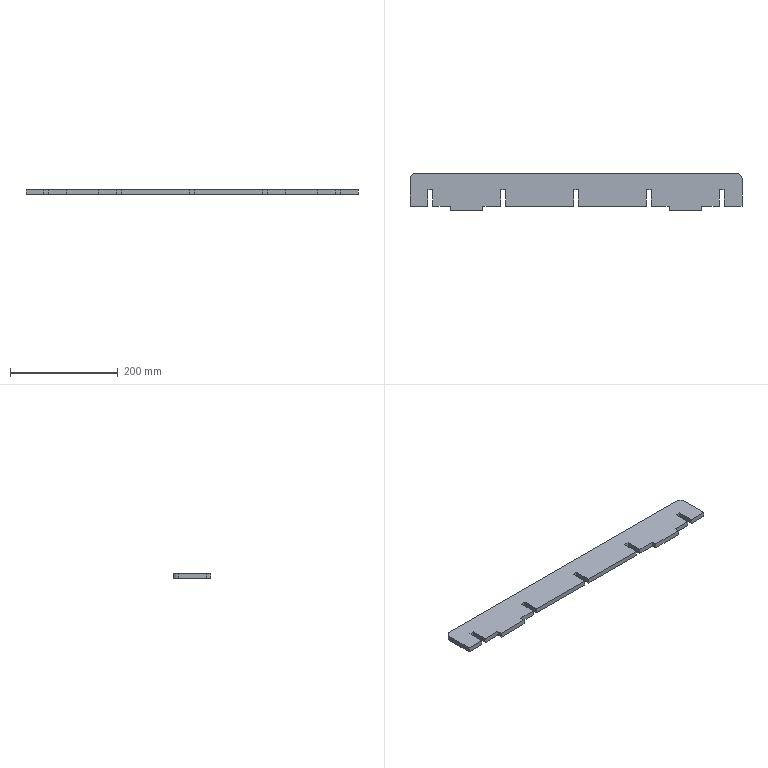Part | SolidWorks | features FlatPattern 1, SMBaseFlange 1, SheetMetal 1 | 1 solid | 36 faces | box 615 x 70 x 9 mm | volume 336641 mm3 | plane 34 | cylinder 2 | commonest cylinder face diameters 20 x2
STEP:
#1=CARTESIAN_POINT('',(336.887,-110.303,0.));
#2=VERTEX_POINT('',#1);
#3=CARTESIAN_POINT('',(369.887,-110.303,0.));
#4=VERTEX_POINT('',#3);
#5=CARTESIAN_POINT('',(336.887,-110.303,0.));
#6=DIRECTION('',(1.,0.,0.));
#7=VECTOR('',#6,1000.);
#8=LINE('',#5,#7);
#9=EDGE_CURVE('',#2,#4,#8,.T.);
#10=ORIENTED_EDGE('',*,*,#9,.F.);
#11=CARTESIAN_POINT('',(336.887,-110.303,-9.));
#12=VERTEX_POINT('',#11);
#13=CARTESIAN_POINT('',(336.887,-110.303,-9.));
#14=DIRECTION('',(0.,0.,1.));
#15=VECTOR('',#14,1000.);
#16=LINE('',#13,#15);
#17=EDGE_CURVE('',#12,#2,#16,.T.);
#18=ORIENTED_EDGE('',*,*,#17,.F.);
#19=CARTESIAN_POINT('',(369.887,-110.303,-9.));
#20=VERTEX_POINT('',#19);
#21=CARTESIAN_POINT('',(336.887,-110.303,-9.));
#22=DIRECTION('',(1.,0.,0.));
#23=VECTOR('',#22,1000.);
#24=LINE('',#21,#23);
#25=EDGE_CURVE('',#12,#20,#24,.T.);
#26=ORIENTED_EDGE('',*,*,#25,.T.);
#27=CARTESIAN_POINT('',(369.887,-110.303,-9.));
#28=DIRECTION('',(0.,0.,1.));
#29=VECTOR('',#28,1000.);
#30=LINE('',#27,#29);
#31=EDGE_CURVE('',#20,#4,#30,.T.);
#32=ORIENTED_EDGE('',*,*,#31,.T.);
#33=EDGE_LOOP('',(#10,#18,#26,#32));
#34=FACE_OUTER_BOUND('',#33,.T.);
#35=CARTESIAN_POINT('',(336.887,-110.303,-9.));
#36=DIRECTION('',(0.,-1.,0.));
#37=DIRECTION('',(1.,0.,0.));
#38=AXIS2_PLACEMENT_3D('',#35,#36,#37);
#39=PLANE('',#38);
#40=ADVANCED_FACE('',(#34),#39,.T.);
#41=CARTESIAN_POINT('',(336.887,-79.303,0.));
#42=VERTEX_POINT('',#41);
#43=CARTESIAN_POINT('',(336.887,-79.303,0.));
#44=DIRECTION('',(0.,-1.,0.));
#45=VECTOR('',#44,1000.);
#46=LINE('',#43,#45);
#47=EDGE_CURVE('',#42,#2,#46,.T.);
#48=ORIENTED_EDGE('',*,*,#47,.F.);
#49=CARTESIAN_POINT('',(336.887,-79.303,-9.));
#50=VERTEX_POINT('',#49);
#51=CARTESIAN_POINT('',(336.887,-79.303,-9.));
#52=DIRECTION('',(0.,0.,1.));
#53=VECTOR('',#52,1000.);
#54=LINE('',#51,#53);
#55=EDGE_CURVE('',#50,#42,#54,.T.);
#56=ORIENTED_EDGE('',*,*,#55,.F.);
#57=CARTESIAN_POINT('',(336.887,-79.303,-9.));
#58=DIRECTION('',(0.,-1.,0.));
#59=VECTOR('',#58,1000.);
#60=LINE('',#57,#59);
#61=EDGE_CURVE('',#50,#12,#60,.T.);
#62=ORIENTED_EDGE('',*,*,#61,.T.);
#63=ORIENTED_EDGE('',*,*,#17,.T.);
#64=EDGE_LOOP('',(#48,#56,#62,#63));
#65=FACE_OUTER_BOUND('',#64,.T.);
#66=CARTESIAN_POINT('',(336.887,-79.303,-9.));
#67=DIRECTION('',(-1.,0.,0.));
#68=DIRECTION('',(0.,0.,1.));
#69=AXIS2_PLACEMENT_3D('',#66,#67,#68);
#70=PLANE('',#69);
#71=ADVANCED_FACE('',(#65),#70,.T.);
#72=CARTESIAN_POINT('',(327.887,-79.303,0.));
#73=VERTEX_POINT('',#72);
#74=CARTESIAN_POINT('',(327.887,-79.303,0.));
#75=DIRECTION('',(1.,0.,0.));
#76=VECTOR('',#75,1000.);
#77=LINE('',#74,#76);
#78=EDGE_CURVE('',#73,#42,#77,.T.);
#79=ORIENTED_EDGE('',*,*,#78,.F.);
#80=CARTESIAN_POINT('',(327.887,-79.303,-9.));
#81=VERTEX_POINT('',#80);
#82=CARTESIAN_POINT('',(327.887,-79.303,-9.));
#83=DIRECTION('',(0.,0.,1.));
#84=VECTOR('',#83,1000.);
#85=LINE('',#82,#84);
#86=EDGE_CURVE('',#81,#73,#85,.T.);
#87=ORIENTED_EDGE('',*,*,#86,.F.);
#88=CARTESIAN_POINT('',(327.887,-79.303,-9.));
#89=DIRECTION('',(1.,0.,0.));
#90=VECTOR('',#89,1000.);
#91=LINE('',#88,#90);
#92=EDGE_CURVE('',#81,#50,#91,.T.);
#93=ORIENTED_EDGE('',*,*,#92,.T.);
#94=ORIENTED_EDGE('',*,*,#55,.T.);
#95=EDGE_LOOP('',(#79,#87,#93,#94));
#96=FACE_OUTER_BOUND('',#95,.T.);
#97=CARTESIAN_POINT('',(327.887,-79.303,-9.));
#98=DIRECTION('',(0.,-1.,0.));
#99=DIRECTION('',(0.,0.,-1.));
#100=AXIS2_PLACEMENT_3D('',#97,#98,#99);
#101=PLANE('',#100);
#102=ADVANCED_FACE('',(#96),#101,.T.);
#103=CARTESIAN_POINT('',(327.887,-110.303,0.));
#104=VERTEX_POINT('',#103);
#105=CARTESIAN_POINT('',(327.887,-110.303,0.));
#106=DIRECTION('',(0.,1.,0.));
#107=VECTOR('',#106,1000.);
#108=LINE('',#105,#107);
#109=EDGE_CURVE('',#104,#73,#108,.T.);
#110=ORIENTED_EDGE('',*,*,#109,.F.);
#111=CARTESIAN_POINT('',(327.887,-110.303,-9.));
#112=VERTEX_POINT('',#111);
#113=CARTESIAN_POINT('',(327.887,-110.303,-9.));
#114=DIRECTION('',(0.,0.,1.));
#115=VECTOR('',#114,1000.);
#116=LINE('',#113,#115);
#117=EDGE_CURVE('',#112,#104,#116,.T.);
#118=ORIENTED_EDGE('',*,*,#117,.F.);
#119=CARTESIAN_POINT('',(327.887,-110.303,-9.));
#120=DIRECTION('',(0.,1.,0.));
#121=VECTOR('',#120,1000.);
#122=LINE('',#119,#121);
#123=EDGE_CURVE('',#112,#81,#122,.T.);
#124=ORIENTED_EDGE('',*,*,#123,.T.);
#125=ORIENTED_EDGE('',*,*,#86,.T.);
#126=EDGE_LOOP('',(#110,#118,#124,#125));
#127=FACE_OUTER_BOUND('',#126,.T.);
#128=CARTESIAN_POINT('',(327.887,-110.303,-9.));
#129=DIRECTION('',(1.,0.,0.));
#130=DIRECTION('',(0.,1.,0.));
#131=AXIS2_PLACEMENT_3D('',#128,#129,#130);
#132=PLANE('',#131);
#133=ADVANCED_FACE('',(#127),#132,.T.);
#134=CARTESIAN_POINT('',(294.887,-110.303,0.));
#135=VERTEX_POINT('',#134);
#136=CARTESIAN_POINT('',(294.887,-110.303,0.));
#137=DIRECTION('',(1.,0.,0.));
#138=VECTOR('',#137,1000.);
#139=LINE('',#136,#138);
#140=EDGE_CURVE('',#135,#104,#139,.T.);
#141=ORIENTED_EDGE('',*,*,#140,.F.);
#142=CARTESIAN_POINT('',(294.887,-110.303,-9.));
#143=VERTEX_POINT('',#142);
#144=CARTESIAN_POINT('',(294.887,-110.303,-9.));
#145=DIRECTION('',(0.,0.,1.));
#146=VECTOR('',#145,1000.);
#147=LINE('',#144,#146);
#148=EDGE_CURVE('',#143,#135,#147,.T.);
#149=ORIENTED_EDGE('',*,*,#148,.F.);
#150=CARTESIAN_POINT('',(294.887,-110.303,-9.));
#151=DIRECTION('',(1.,0.,0.));
#152=VECTOR('',#151,1000.);
#153=LINE('',#150,#152);
#154=EDGE_CURVE('',#143,#112,#153,.T.);
#155=ORIENTED_EDGE('',*,*,#154,.T.);
#156=ORIENTED_EDGE('',*,*,#117,.T.);
#157=EDGE_LOOP('',(#141,#149,#155,#156));
#158=FACE_OUTER_BOUND('',#157,.T.);
#159=CARTESIAN_POINT('',(294.887,-110.303,-9.));
#160=DIRECTION('',(0.,-1.,0.));
#161=DIRECTION('',(1.,0.,0.));
#162=AXIS2_PLACEMENT_3D('',#159,#160,#161);
#163=PLANE('',#162);
#164=ADVANCED_FACE('',(#158),#163,.T.);
#165=CARTESIAN_POINT('',(294.887,-118.803,0.));
#166=VERTEX_POINT('',#165);
#167=CARTESIAN_POINT('',(294.887,-118.803,0.));
#168=DIRECTION('',(0.,1.,0.));
#169=VECTOR('',#168,1000.);
#170=LINE('',#167,#169);
#171=EDGE_CURVE('',#166,#135,#170,.T.);
#172=ORIENTED_EDGE('',*,*,#171,.F.);
#173=CARTESIAN_POINT('',(294.887,-118.803,-9.));
#174=VERTEX_POINT('',#173);
#175=CARTESIAN_POINT('',(294.887,-118.803,-9.));
#176=DIRECTION('',(0.,0.,1.));
#177=VECTOR('',#176,1000.);
#178=LINE('',#175,#177);
#179=EDGE_CURVE('',#174,#166,#178,.T.);
#180=ORIENTED_EDGE('',*,*,#179,.F.);
#181=CARTESIAN_POINT('',(294.887,-118.803,-9.));
#182=DIRECTION('',(0.,1.,0.));
#183=VECTOR('',#182,1000.);
#184=LINE('',#181,#183);
#185=EDGE_CURVE('',#174,#143,#184,.T.);
#186=ORIENTED_EDGE('',*,*,#185,.T.);
#187=ORIENTED_EDGE('',*,*,#148,.T.);
#188=EDGE_LOOP('',(#172,#180,#186,#187));
#189=FACE_OUTER_BOUND('',#188,.T.);
#190=CARTESIAN_POINT('',(294.887,-118.803,-9.));
#191=DIRECTION('',(1.,0.,0.));
#192=DIRECTION('',(0.,0.,-1.));
#193=AXIS2_PLACEMENT_3D('',#190,#191,#192);
#194=PLANE('',#193);
#195=ADVANCED_FACE('',(#189),#194,.T.);
#196=CARTESIAN_POINT('',(234.887,-118.803,0.));
#197=VERTEX_POINT('',#196);
#198=CARTESIAN_POINT('',(234.887,-118.803,0.));
#199=DIRECTION('',(1.,0.,0.));
#200=VECTOR('',#199,1000.);
#201=LINE('',#198,#200);
#202=EDGE_CURVE('',#197,#166,#201,.T.);
#203=ORIENTED_EDGE('',*,*,#202,.F.);
#204=CARTESIAN_POINT('',(234.887,-118.803,-9.));
#205=VERTEX_POINT('',#204);
#206=CARTESIAN_POINT('',(234.887,-118.803,-9.));
#207=DIRECTION('',(0.,0.,1.));
#208=VECTOR('',#207,1000.);
#209=LINE('',#206,#208);
#210=EDGE_CURVE('',#205,#197,#209,.T.);
#211=ORIENTED_EDGE('',*,*,#210,.F.);
#212=CARTESIAN_POINT('',(234.887,-118.803,-9.));
#213=DIRECTION('',(1.,0.,0.));
#214=VECTOR('',#213,1000.);
#215=LINE('',#212,#214);
#216=EDGE_CURVE('',#205,#174,#215,.T.);
#217=ORIENTED_EDGE('',*,*,#216,.T.);
#218=ORIENTED_EDGE('',*,*,#179,.T.);
#219=EDGE_LOOP('',(#203,#211,#217,#218));
#220=FACE_OUTER_BOUND('',#219,.T.);
#221=CARTESIAN_POINT('',(234.887,-118.803,-9.));
#222=DIRECTION('',(0.,-1.,0.));
#223=DIRECTION('',(0.,0.,-1.));
#224=AXIS2_PLACEMENT_3D('',#221,#222,#223);
#225=PLANE('',#224);
#226=ADVANCED_FACE('',(#220),#225,.T.);
#227=CARTESIAN_POINT('',(234.887,-110.303,0.));
#228=VERTEX_POINT('',#227);
#229=CARTESIAN_POINT('',(234.887,-110.303,0.));
#230=DIRECTION('',(0.,-1.,0.));
#231=VECTOR('',#230,1000.);
#232=LINE('',#229,#231);
#233=EDGE_CURVE('',#228,#197,#232,.T.);
#234=ORIENTED_EDGE('',*,*,#233,.F.);
#235=CARTESIAN_POINT('',(234.887,-110.303,-9.));
#236=VERTEX_POINT('',#235);
#237=CARTESIAN_POINT('',(234.887,-110.303,-9.));
#238=DIRECTION('',(0.,0.,1.));
#239=VECTOR('',#238,1000.);
#240=LINE('',#237,#239);
#241=EDGE_CURVE('',#236,#228,#240,.T.);
#242=ORIENTED_EDGE('',*,*,#241,.F.);
#243=CARTESIAN_POINT('',(234.887,-110.303,-9.));
#244=DIRECTION('',(0.,-1.,0.));
#245=VECTOR('',#244,1000.);
#246=LINE('',#243,#245);
#247=EDGE_CURVE('',#236,#205,#246,.T.);
#248=ORIENTED_EDGE('',*,*,#247,.T.);
#249=ORIENTED_EDGE('',*,*,#210,.T.);
#250=EDGE_LOOP('',(#234,#242,#248,#249));
#251=FACE_OUTER_BOUND('',#250,.T.);
#252=CARTESIAN_POINT('',(234.887,-110.303,-9.));
#253=DIRECTION('',(-1.,0.,0.));
#254=DIRECTION('',(0.,-1.,0.));
#255=AXIS2_PLACEMENT_3D('',#252,#253,#254);
#256=PLANE('',#255);
#257=ADVANCED_FACE('',(#251),#256,.T.);
#258=CARTESIAN_POINT('',(201.887,-110.303,0.));
#259=VERTEX_POINT('',#258);
#260=CARTESIAN_POINT('',(201.887,-110.303,0.));
#261=DIRECTION('',(1.,0.,0.));
#262=VECTOR('',#261,1000.);
#263=LINE('',#260,#262);
#264=EDGE_CURVE('',#259,#228,#263,.T.);
#265=ORIENTED_EDGE('',*,*,#264,.F.);
#266=CARTESIAN_POINT('',(201.887,-110.303,-9.));
#267=VERTEX_POINT('',#266);
#268=CARTESIAN_POINT('',(201.887,-110.303,-9.));
#269=DIRECTION('',(0.,0.,1.));
#270=VECTOR('',#269,1000.);
#271=LINE('',#268,#270);
#272=EDGE_CURVE('',#267,#259,#271,.T.);
#273=ORIENTED_EDGE('',*,*,#272,.F.);
#274=CARTESIAN_POINT('',(201.887,-110.303,-9.));
#275=DIRECTION('',(1.,0.,0.));
#276=VECTOR('',#275,1000.);
#277=LINE('',#274,#276);
#278=EDGE_CURVE('',#267,#236,#277,.T.);
#279=ORIENTED_EDGE('',*,*,#278,.T.);
#280=ORIENTED_EDGE('',*,*,#241,.T.);
#281=EDGE_LOOP('',(#265,#273,#279,#280));
#282=FACE_OUTER_BOUND('',#281,.T.);
#283=CARTESIAN_POINT('',(201.887,-110.303,-9.));
#284=DIRECTION('',(0.,-1.,0.));
#285=DIRECTION('',(1.,0.,0.));
#286=AXIS2_PLACEMENT_3D('',#283,#284,#285);
#287=PLANE('',#286);
#288=ADVANCED_FACE('',(#282),#287,.T.);
#289=CARTESIAN_POINT('',(201.887,-79.303,0.));
#290=VERTEX_POINT('',#289);
#291=CARTESIAN_POINT('',(201.887,-79.303,0.));
#292=DIRECTION('',(0.,-1.,0.));
#293=VECTOR('',#292,1000.);
#294=LINE('',#291,#293);
#295=EDGE_CURVE('',#290,#259,#294,.T.);
#296=ORIENTED_EDGE('',*,*,#295,.F.);
#297=CARTESIAN_POINT('',(201.887,-79.303,-9.));
#298=VERTEX_POINT('',#297);
#299=CARTESIAN_POINT('',(201.887,-79.303,-9.));
#300=DIRECTION('',(0.,0.,1.));
#301=VECTOR('',#300,1000.);
#302=LINE('',#299,#301);
#303=EDGE_CURVE('',#298,#290,#302,.T.);
#304=ORIENTED_EDGE('',*,*,#303,.F.);
#305=CARTESIAN_POINT('',(201.887,-79.303,-9.));
#306=DIRECTION('',(0.,-1.,0.));
#307=VECTOR('',#306,1000.);
#308=LINE('',#305,#307);
#309=EDGE_CURVE('',#298,#267,#308,.T.);
#310=ORIENTED_EDGE('',*,*,#309,.T.);
#311=ORIENTED_EDGE('',*,*,#272,.T.);
#312=EDGE_LOOP('',(#296,#304,#310,#311));
#313=FACE_OUTER_BOUND('',#312,.T.);
#314=CARTESIAN_POINT('',(201.887,-79.303,-9.));
#315=DIRECTION('',(-1.,0.,0.));
#316=DIRECTION('',(0.,0.,1.));
#317=AXIS2_PLACEMENT_3D('',#314,#315,#316);
#318=PLANE('',#317);
#319=ADVANCED_FACE('',(#313),#318,.T.);
#320=CARTESIAN_POINT('',(192.887,-79.303,0.));
#321=VERTEX_POINT('',#320);
#322=CARTESIAN_POINT('',(192.887,-79.303,0.));
#323=DIRECTION('',(1.,0.,0.));
#324=VECTOR('',#323,1000.);
#325=LINE('',#322,#324);
#326=EDGE_CURVE('',#321,#290,#325,.T.);
#327=ORIENTED_EDGE('',*,*,#326,.F.);
#328=CARTESIAN_POINT('',(192.887,-79.303,-9.));
#329=VERTEX_POINT('',#328);
#330=CARTESIAN_POINT('',(192.887,-79.303,-9.));
#331=DIRECTION('',(0.,0.,1.));
#332=VECTOR('',#331,1000.);
#333=LINE('',#330,#332);
#334=EDGE_CURVE('',#329,#321,#333,.T.);
#335=ORIENTED_EDGE('',*,*,#334,.F.);
#336=CARTESIAN_POINT('',(192.887,-79.303,-9.));
#337=DIRECTION('',(1.,0.,0.));
#338=VECTOR('',#337,1000.);
#339=LINE('',#336,#338);
#340=EDGE_CURVE('',#329,#298,#339,.T.);
#341=ORIENTED_EDGE('',*,*,#340,.T.);
#342=ORIENTED_EDGE('',*,*,#303,.T.);
#343=EDGE_LOOP('',(#327,#335,#341,#342));
#344=FACE_OUTER_BOUND('',#343,.T.);
#345=CARTESIAN_POINT('',(192.887,-79.303,-9.));
#346=DIRECTION('',(0.,-1.,0.));
#347=DIRECTION('',(0.,0.,-1.));
#348=AXIS2_PLACEMENT_3D('',#345,#346,#347);
#349=PLANE('',#348);
#350=ADVANCED_FACE('',(#344),#349,.T.);
#351=CARTESIAN_POINT('',(192.887,-110.303,0.));
#352=VERTEX_POINT('',#351);
#353=CARTESIAN_POINT('',(192.887,-110.303,0.));
#354=DIRECTION('',(0.,1.,0.));
#355=VECTOR('',#354,1000.);
#356=LINE('',#353,#355);
#357=EDGE_CURVE('',#352,#321,#356,.T.);
#358=ORIENTED_EDGE('',*,*,#357,.F.);
#359=CARTESIAN_POINT('',(192.887,-110.303,-9.));
#360=VERTEX_POINT('',#359);
#361=CARTESIAN_POINT('',(192.887,-110.303,-9.));
#362=DIRECTION('',(0.,0.,1.));
#363=VECTOR('',#362,1000.);
#364=LINE('',#361,#363);
#365=EDGE_CURVE('',#360,#352,#364,.T.);
#366=ORIENTED_EDGE('',*,*,#365,.F.);
#367=CARTESIAN_POINT('',(192.887,-110.303,-9.));
#368=DIRECTION('',(0.,1.,0.));
#369=VECTOR('',#368,1000.);
#370=LINE('',#367,#369);
#371=EDGE_CURVE('',#360,#329,#370,.T.);
#372=ORIENTED_EDGE('',*,*,#371,.T.);
#373=ORIENTED_EDGE('',*,*,#334,.T.);
#374=EDGE_LOOP('',(#358,#366,#372,#373));
#375=FACE_OUTER_BOUND('',#374,.T.);
#376=CARTESIAN_POINT('',(192.887,-110.303,-9.));
#377=DIRECTION('',(1.,0.,0.));
#378=DIRECTION('',(0.,1.,0.));
#379=AXIS2_PLACEMENT_3D('',#376,#377,#378);
#380=PLANE('',#379);
#381=ADVANCED_FACE('',(#375),#380,.T.);
#382=CARTESIAN_POINT('',(66.887,-110.303,0.));
#383=VERTEX_POINT('',#382);
#384=CARTESIAN_POINT('',(66.887,-110.303,0.));
#385=DIRECTION('',(1.,0.,0.));
#386=VECTOR('',#385,1000.);
#387=LINE('',#384,#386);
#388=EDGE_CURVE('',#383,#352,#387,.T.);
#389=ORIENTED_EDGE('',*,*,#388,.F.);
#390=CARTESIAN_POINT('',(66.887,-110.303,-9.));
#391=VERTEX_POINT('',#390);
#392=CARTESIAN_POINT('',(66.887,-110.303,-9.));
#393=DIRECTION('',(0.,0.,1.));
#394=VECTOR('',#393,1000.);
#395=LINE('',#392,#394);
#396=EDGE_CURVE('',#391,#383,#395,.T.);
#397=ORIENTED_EDGE('',*,*,#396,.F.);
#398=CARTESIAN_POINT('',(66.887,-110.303,-9.));
#399=DIRECTION('',(1.,0.,0.));
#400=VECTOR('',#399,1000.);
#401=LINE('',#398,#400);
#402=EDGE_CURVE('',#391,#360,#401,.T.);
#403=ORIENTED_EDGE('',*,*,#402,.T.);
#404=ORIENTED_EDGE('',*,*,#365,.T.);
#405=EDGE_LOOP('',(#389,#397,#403,#404));
#406=FACE_OUTER_BOUND('',#405,.T.);
#407=CARTESIAN_POINT('',(66.887,-110.303,-9.));
#408=DIRECTION('',(0.,-1.,0.));
#409=DIRECTION('',(1.,0.,0.));
#410=AXIS2_PLACEMENT_3D('',#407,#408,#409);
#411=PLANE('',#410);
#412=ADVANCED_FACE('',(#406),#411,.T.);
#413=CARTESIAN_POINT('',(66.887,-79.303,0.));
#414=VERTEX_POINT('',#413);
#415=CARTESIAN_POINT('',(66.887,-79.303,0.));
#416=DIRECTION('',(0.,-1.,0.));
#417=VECTOR('',#416,1000.);
#418=LINE('',#415,#417);
#419=EDGE_CURVE('',#414,#383,#418,.T.);
#420=ORIENTED_EDGE('',*,*,#419,.F.);
#421=CARTESIAN_POINT('',(66.887,-79.303,-9.));
#422=VERTEX_POINT('',#421);
#423=CARTESIAN_POINT('',(66.887,-79.303,-9.));
#424=DIRECTION('',(0.,0.,1.));
#425=VECTOR('',#424,1000.);
#426=LINE('',#423,#425);
#427=EDGE_CURVE('',#422,#414,#426,.T.);
#428=ORIENTED_EDGE('',*,*,#427,.F.);
#429=CARTESIAN_POINT('',(66.887,-79.303,-9.));
#430=DIRECTION('',(0.,-1.,0.));
#431=VECTOR('',#430,1000.);
#432=LINE('',#429,#431);
#433=EDGE_CURVE('',#422,#391,#432,.T.);
#434=ORIENTED_EDGE('',*,*,#433,.T.);
#435=ORIENTED_EDGE('',*,*,#396,.T.);
#436=EDGE_LOOP('',(#420,#428,#434,#435));
#437=FACE_OUTER_BOUND('',#436,.T.);
#438=CARTESIAN_POINT('',(66.887,-79.303,-9.));
#439=DIRECTION('',(-1.,0.,0.));
#440=DIRECTION('',(0.,0.,1.));
#441=AXIS2_PLACEMENT_3D('',#438,#439,#440);
#442=PLANE('',#441);
#443=ADVANCED_FACE('',(#437),#442,.T.);
#444=CARTESIAN_POINT('',(57.887,-79.303,0.));
#445=VERTEX_POINT('',#444);
#446=CARTESIAN_POINT('',(57.887,-79.303,0.));
#447=DIRECTION('',(1.,0.,0.));
#448=VECTOR('',#447,1000.);
#449=LINE('',#446,#448);
#450=EDGE_CURVE('',#445,#414,#449,.T.);
#451=ORIENTED_EDGE('',*,*,#450,.F.);
#452=CARTESIAN_POINT('',(57.887,-79.303,-9.));
#453=VERTEX_POINT('',#452);
#454=CARTESIAN_POINT('',(57.887,-79.303,-9.));
#455=DIRECTION('',(0.,0.,1.));
#456=VECTOR('',#455,1000.);
#457=LINE('',#454,#456);
#458=EDGE_CURVE('',#453,#445,#457,.T.);
#459=ORIENTED_EDGE('',*,*,#458,.F.);
#460=CARTESIAN_POINT('',(57.887,-79.303,-9.));
#461=DIRECTION('',(1.,0.,0.));
#462=VECTOR('',#461,1000.);
#463=LINE('',#460,#462);
#464=EDGE_CURVE('',#453,#422,#463,.T.);
#465=ORIENTED_EDGE('',*,*,#464,.T.);
#466=ORIENTED_EDGE('',*,*,#427,.T.);
#467=EDGE_LOOP('',(#451,#459,#465,#466));
#468=FACE_OUTER_BOUND('',#467,.T.);
#469=CARTESIAN_POINT('',(57.887,-79.303,-9.));
#470=DIRECTION('',(0.,-1.,0.));
#471=DIRECTION('',(0.,0.,-1.));
#472=AXIS2_PLACEMENT_3D('',#469,#470,#471);
#473=PLANE('',#472);
#474=ADVANCED_FACE('',(#468),#473,.T.);
#475=CARTESIAN_POINT('',(57.887,-110.303,0.));
#476=VERTEX_POINT('',#475);
#477=CARTESIAN_POINT('',(57.887,-110.303,0.));
#478=DIRECTION('',(0.,1.,0.));
#479=VECTOR('',#478,1000.);
#480=LINE('',#477,#479);
#481=EDGE_CURVE('',#476,#445,#480,.T.);
#482=ORIENTED_EDGE('',*,*,#481,.F.);
#483=CARTESIAN_POINT('',(57.887,-110.303,-9.));
#484=VERTEX_POINT('',#483);
#485=CARTESIAN_POINT('',(57.887,-110.303,-9.));
#486=DIRECTION('',(0.,0.,1.));
#487=VECTOR('',#486,1000.);
#488=LINE('',#485,#487);
#489=EDGE_CURVE('',#484,#476,#488,.T.);
#490=ORIENTED_EDGE('',*,*,#489,.F.);
#491=CARTESIAN_POINT('',(57.887,-110.303,-9.));
#492=DIRECTION('',(0.,1.,0.));
#493=VECTOR('',#492,1000.);
#494=LINE('',#491,#493);
#495=EDGE_CURVE('',#484,#453,#494,.T.);
#496=ORIENTED_EDGE('',*,*,#495,.T.);
#497=ORIENTED_EDGE('',*,*,#458,.T.);
#498=EDGE_LOOP('',(#482,#490,#496,#497));
#499=FACE_OUTER_BOUND('',#498,.T.);
#500=CARTESIAN_POINT('',(57.887,-110.303,-9.));
#501=DIRECTION('',(1.,0.,0.));
#502=DIRECTION('',(0.,0.,-1.));
#503=AXIS2_PLACEMENT_3D('',#500,#501,#502);
#504=PLANE('',#503);
#505=ADVANCED_FACE('',(#499),#504,.T.);
#506=CARTESIAN_POINT('',(-68.113,-110.303,0.));
#507=VERTEX_POINT('',#506);
#508=CARTESIAN_POINT('',(-68.113,-110.303,0.));
#509=DIRECTION('',(1.,0.,0.));
#510=VECTOR('',#509,1000.);
#511=LINE('',#508,#510);
#512=EDGE_CURVE('',#507,#476,#511,.T.);
#513=ORIENTED_EDGE('',*,*,#512,.F.);
#514=CARTESIAN_POINT('',(-68.113,-110.303,-9.));
#515=VERTEX_POINT('',#514);
#516=CARTESIAN_POINT('',(-68.113,-110.303,-9.));
#517=DIRECTION('',(0.,0.,1.));
#518=VECTOR('',#517,1000.);
#519=LINE('',#516,#518);
#520=EDGE_CURVE('',#515,#507,#519,.T.);
#521=ORIENTED_EDGE('',*,*,#520,.F.);
#522=CARTESIAN_POINT('',(-68.113,-110.303,-9.));
#523=DIRECTION('',(1.,0.,0.));
#524=VECTOR('',#523,1000.);
#525=LINE('',#522,#524);
#526=EDGE_CURVE('',#515,#484,#525,.T.);
#527=ORIENTED_EDGE('',*,*,#526,.T.);
#528=ORIENTED_EDGE('',*,*,#489,.T.);
#529=EDGE_LOOP('',(#513,#521,#527,#528));
#530=FACE_OUTER_BOUND('',#529,.T.);
#531=CARTESIAN_POINT('',(-68.113,-110.303,-9.));
#532=DIRECTION('',(0.,-1.,0.));
#533=DIRECTION('',(1.,0.,0.));
#534=AXIS2_PLACEMENT_3D('',#531,#532,#533);
#535=PLANE('',#534);
#536=ADVANCED_FACE('',(#530),#535,.T.);
#537=CARTESIAN_POINT('',(-68.113,-79.303,0.));
#538=VERTEX_POINT('',#537);
#539=CARTESIAN_POINT('',(-68.113,-79.303,0.));
#540=DIRECTION('',(0.,-1.,0.));
#541=VECTOR('',#540,1000.);
#542=LINE('',#539,#541);
#543=EDGE_CURVE('',#538,#507,#542,.T.);
#544=ORIENTED_EDGE('',*,*,#543,.F.);
#545=CARTESIAN_POINT('',(-68.113,-79.303,-9.));
#546=VERTEX_POINT('',#545);
#547=CARTESIAN_POINT('',(-68.113,-79.303,-9.));
#548=DIRECTION('',(0.,0.,1.));
#549=VECTOR('',#548,1000.);
#550=LINE('',#547,#549);
#551=EDGE_CURVE('',#546,#538,#550,.T.);
#552=ORIENTED_EDGE('',*,*,#551,.F.);
#553=CARTESIAN_POINT('',(-68.113,-79.303,-9.));
#554=DIRECTION('',(0.,-1.,0.));
#555=VECTOR('',#554,1000.);
#556=LINE('',#553,#555);
#557=EDGE_CURVE('',#546,#515,#556,.T.);
#558=ORIENTED_EDGE('',*,*,#557,.T.);
#559=ORIENTED_EDGE('',*,*,#520,.T.);
#560=EDGE_LOOP('',(#544,#552,#558,#559));
#561=FACE_OUTER_BOUND('',#560,.T.);
#562=CARTESIAN_POINT('',(-68.113,-79.303,-9.));
#563=DIRECTION('',(-1.,0.,0.));
#564=DIRECTION('',(0.,0.,1.));
#565=AXIS2_PLACEMENT_3D('',#562,#563,#564);
#566=PLANE('',#565);
#567=ADVANCED_FACE('',(#561),#566,.T.);
#568=CARTESIAN_POINT('',(-77.113,-79.303,0.));
#569=VERTEX_POINT('',#568);
#570=CARTESIAN_POINT('',(-77.113,-79.303,0.));
#571=DIRECTION('',(1.,0.,0.));
#572=VECTOR('',#571,1000.);
#573=LINE('',#570,#572);
#574=EDGE_CURVE('',#569,#538,#573,.T.);
#575=ORIENTED_EDGE('',*,*,#574,.F.);
#576=CARTESIAN_POINT('',(-77.113,-79.303,-9.));
#577=VERTEX_POINT('',#576);
#578=CARTESIAN_POINT('',(-77.113,-79.303,-9.));
#579=DIRECTION('',(0.,0.,1.));
#580=VECTOR('',#579,1000.);
#581=LINE('',#578,#580);
#582=EDGE_CURVE('',#577,#569,#581,.T.);
#583=ORIENTED_EDGE('',*,*,#582,.F.);
#584=CARTESIAN_POINT('',(-77.113,-79.303,-9.));
#585=DIRECTION('',(1.,0.,0.));
#586=VECTOR('',#585,1000.);
#587=LINE('',#584,#586);
#588=EDGE_CURVE('',#577,#546,#587,.T.);
#589=ORIENTED_EDGE('',*,*,#588,.T.);
#590=ORIENTED_EDGE('',*,*,#551,.T.);
#591=EDGE_LOOP('',(#575,#583,#589,#590));
#592=FACE_OUTER_BOUND('',#591,.T.);
#593=CARTESIAN_POINT('',(-77.113,-79.303,-9.));
#594=DIRECTION('',(0.,-1.,0.));
#595=DIRECTION('',(0.,0.,-1.));
#596=AXIS2_PLACEMENT_3D('',#593,#594,#595);
#597=PLANE('',#596);
#598=ADVANCED_FACE('',(#592),#597,.T.);
#599=CARTESIAN_POINT('',(-77.113,-110.303,0.));
#600=VERTEX_POINT('',#599);
#601=CARTESIAN_POINT('',(-77.113,-110.303,0.));
#602=DIRECTION('',(0.,1.,0.));
#603=VECTOR('',#602,1000.);
#604=LINE('',#601,#603);
#605=EDGE_CURVE('',#600,#569,#604,.T.);
#606=ORIENTED_EDGE('',*,*,#605,.F.);
#607=CARTESIAN_POINT('',(-77.113,-110.303,-9.));
#608=VERTEX_POINT('',#607);
#609=CARTESIAN_POINT('',(-77.113,-110.303,-9.));
#610=DIRECTION('',(0.,0.,1.));
#611=VECTOR('',#610,1000.);
#612=LINE('',#609,#611);
#613=EDGE_CURVE('',#608,#600,#612,.T.);
#614=ORIENTED_EDGE('',*,*,#613,.F.);
#615=CARTESIAN_POINT('',(-77.113,-110.303,-9.));
#616=DIRECTION('',(0.,1.,0.));
#617=VECTOR('',#616,1000.);
#618=LINE('',#615,#617);
#619=EDGE_CURVE('',#608,#577,#618,.T.);
#620=ORIENTED_EDGE('',*,*,#619,.T.);
#621=ORIENTED_EDGE('',*,*,#582,.T.);
#622=EDGE_LOOP('',(#606,#614,#620,#621));
#623=FACE_OUTER_BOUND('',#622,.T.);
#624=CARTESIAN_POINT('',(-77.113,-110.303,-9.));
#625=DIRECTION('',(1.,0.,0.));
#626=DIRECTION('',(0.,1.,0.));
#627=AXIS2_PLACEMENT_3D('',#624,#625,#626);
#628=PLANE('',#627);
#629=ADVANCED_FACE('',(#623),#628,.T.);
#630=CARTESIAN_POINT('',(-110.113,-110.303,0.));
#631=VERTEX_POINT('',#630);
#632=CARTESIAN_POINT('',(-110.113,-110.303,0.));
#633=DIRECTION('',(1.,0.,0.));
#634=VECTOR('',#633,1000.);
#635=LINE('',#632,#634);
#636=EDGE_CURVE('',#631,#600,#635,.T.);
#637=ORIENTED_EDGE('',*,*,#636,.F.);
#638=CARTESIAN_POINT('',(-110.113,-110.303,-9.));
#639=VERTEX_POINT('',#638);
#640=CARTESIAN_POINT('',(-110.113,-110.303,-9.));
#641=DIRECTION('',(0.,0.,1.));
#642=VECTOR('',#641,1000.);
#643=LINE('',#640,#642);
#644=EDGE_CURVE('',#639,#631,#643,.T.);
#645=ORIENTED_EDGE('',*,*,#644,.F.);
#646=CARTESIAN_POINT('',(-110.113,-110.303,-9.));
#647=DIRECTION('',(1.,0.,0.));
#648=VECTOR('',#647,1000.);
#649=LINE('',#646,#648);
#650=EDGE_CURVE('',#639,#608,#649,.T.);
#651=ORIENTED_EDGE('',*,*,#650,.T.);
#652=ORIENTED_EDGE('',*,*,#613,.T.);
#653=EDGE_LOOP('',(#637,#645,#651,#652));
#654=FACE_OUTER_BOUND('',#653,.T.);
#655=CARTESIAN_POINT('',(-110.113,-110.303,-9.));
#656=DIRECTION('',(0.,-1.,0.));
#657=DIRECTION('',(1.,0.,0.));
#658=AXIS2_PLACEMENT_3D('',#655,#656,#657);
#659=PLANE('',#658);
#660=ADVANCED_FACE('',(#654),#659,.T.);
#661=CARTESIAN_POINT('',(-110.113,-118.803,0.));
#662=VERTEX_POINT('',#661);
#663=CARTESIAN_POINT('',(-110.113,-118.803,0.));
#664=DIRECTION('',(0.,1.,0.));
#665=VECTOR('',#664,1000.);
#666=LINE('',#663,#665);
#667=EDGE_CURVE('',#662,#631,#666,.T.);
#668=ORIENTED_EDGE('',*,*,#667,.F.);
#669=CARTESIAN_POINT('',(-110.113,-118.803,-9.));
#670=VERTEX_POINT('',#669);
#671=CARTESIAN_POINT('',(-110.113,-118.803,-9.));
#672=DIRECTION('',(0.,0.,1.));
#673=VECTOR('',#672,1000.);
#674=LINE('',#671,#673);
#675=EDGE_CURVE('',#670,#662,#674,.T.);
#676=ORIENTED_EDGE('',*,*,#675,.F.);
#677=CARTESIAN_POINT('',(-110.113,-118.803,-9.));
#678=DIRECTION('',(0.,1.,0.));
#679=VECTOR('',#678,1000.);
#680=LINE('',#677,#679);
#681=EDGE_CURVE('',#670,#639,#680,.T.);
#682=ORIENTED_EDGE('',*,*,#681,.T.);
#683=ORIENTED_EDGE('',*,*,#644,.T.);
#684=EDGE_LOOP('',(#668,#676,#682,#683));
#685=FACE_OUTER_BOUND('',#684,.T.);
#686=CARTESIAN_POINT('',(-110.113,-118.803,-9.));
#687=DIRECTION('',(1.,0.,0.));
#688=DIRECTION('',(0.,0.,-1.));
#689=AXIS2_PLACEMENT_3D('',#686,#687,#688);
#690=PLANE('',#689);
#691=ADVANCED_FACE('',(#685),#690,.T.);
#692=CARTESIAN_POINT('',(-170.113,-118.803,0.));
#693=VERTEX_POINT('',#692);
#694=CARTESIAN_POINT('',(-170.113,-118.803,0.));
#695=DIRECTION('',(1.,0.,0.));
#696=VECTOR('',#695,1000.);
#697=LINE('',#694,#696);
#698=EDGE_CURVE('',#693,#662,#697,.T.);
#699=ORIENTED_EDGE('',*,*,#698,.F.);
#700=CARTESIAN_POINT('',(-170.113,-118.803,-9.));
#701=VERTEX_POINT('',#700);
#702=CARTESIAN_POINT('',(-170.113,-118.803,-9.));
#703=DIRECTION('',(0.,0.,1.));
#704=VECTOR('',#703,1000.);
#705=LINE('',#702,#704);
#706=EDGE_CURVE('',#701,#693,#705,.T.);
#707=ORIENTED_EDGE('',*,*,#706,.F.);
#708=CARTESIAN_POINT('',(-170.113,-118.803,-9.));
#709=DIRECTION('',(1.,0.,0.));
#710=VECTOR('',#709,1000.);
#711=LINE('',#708,#710);
#712=EDGE_CURVE('',#701,#670,#711,.T.);
#713=ORIENTED_EDGE('',*,*,#712,.T.);
#714=ORIENTED_EDGE('',*,*,#675,.T.);
#715=EDGE_LOOP('',(#699,#707,#713,#714));
#716=FACE_OUTER_BOUND('',#715,.T.);
#717=CARTESIAN_POINT('',(-170.113,-118.803,-9.));
#718=DIRECTION('',(0.,-1.,0.));
#719=DIRECTION('',(0.,0.,-1.));
#720=AXIS2_PLACEMENT_3D('',#717,#718,#719);
#721=PLANE('',#720);
#722=ADVANCED_FACE('',(#716),#721,.T.);
#723=CARTESIAN_POINT('',(-170.113,-110.303,0.));
#724=VERTEX_POINT('',#723);
#725=CARTESIAN_POINT('',(-170.113,-110.303,0.));
#726=DIRECTION('',(0.,-1.,0.));
#727=VECTOR('',#726,1000.);
#728=LINE('',#725,#727);
#729=EDGE_CURVE('',#724,#693,#728,.T.);
#730=ORIENTED_EDGE('',*,*,#729,.F.);
#731=CARTESIAN_POINT('',(-170.113,-110.303,-9.));
#732=VERTEX_POINT('',#731);
#733=CARTESIAN_POINT('',(-170.113,-110.303,-9.));
#734=DIRECTION('',(0.,0.,1.));
#735=VECTOR('',#734,1000.);
#736=LINE('',#733,#735);
#737=EDGE_CURVE('',#732,#724,#736,.T.);
#738=ORIENTED_EDGE('',*,*,#737,.F.);
#739=CARTESIAN_POINT('',(-170.113,-110.303,-9.));
#740=DIRECTION('',(0.,-1.,0.));
#741=VECTOR('',#740,1000.);
#742=LINE('',#739,#741);
#743=EDGE_CURVE('',#732,#701,#742,.T.);
#744=ORIENTED_EDGE('',*,*,#743,.T.);
#745=ORIENTED_EDGE('',*,*,#706,.T.);
#746=EDGE_LOOP('',(#730,#738,#744,#745));
#747=FACE_OUTER_BOUND('',#746,.T.);
#748=CARTESIAN_POINT('',(-170.113,-110.303,-9.));
#749=DIRECTION('',(-1.,0.,0.));
#750=DIRECTION('',(0.,0.,1.));
#751=AXIS2_PLACEMENT_3D('',#748,#749,#750);
#752=PLANE('',#751);
#753=ADVANCED_FACE('',(#747),#752,.T.);
#754=CARTESIAN_POINT('',(-203.113,-110.303,0.));
#755=VERTEX_POINT('',#754);
#756=CARTESIAN_POINT('',(-203.113,-110.303,0.));
#757=DIRECTION('',(1.,0.,0.));
#758=VECTOR('',#757,1000.);
#759=LINE('',#756,#758);
#760=EDGE_CURVE('',#755,#724,#759,.T.);
#761=ORIENTED_EDGE('',*,*,#760,.F.);
#762=CARTESIAN_POINT('',(-203.113,-110.303,-9.));
#763=VERTEX_POINT('',#762);
#764=CARTESIAN_POINT('',(-203.113,-110.303,-9.));
#765=DIRECTION('',(0.,0.,1.));
#766=VECTOR('',#765,1000.);
#767=LINE('',#764,#766);
#768=EDGE_CURVE('',#763,#755,#767,.T.);
#769=ORIENTED_EDGE('',*,*,#768,.F.);
#770=CARTESIAN_POINT('',(-203.113,-110.303,-9.));
#771=DIRECTION('',(1.,0.,0.));
#772=VECTOR('',#771,1000.);
#773=LINE('',#770,#772);
#774=EDGE_CURVE('',#763,#732,#773,.T.);
#775=ORIENTED_EDGE('',*,*,#774,.T.);
#776=ORIENTED_EDGE('',*,*,#737,.T.);
#777=EDGE_LOOP('',(#761,#769,#775,#776));
#778=FACE_OUTER_BOUND('',#777,.T.);
#779=CARTESIAN_POINT('',(-203.113,-110.303,-9.));
#780=DIRECTION('',(0.,-1.,0.));
#781=DIRECTION('',(1.,0.,0.));
#782=AXIS2_PLACEMENT_3D('',#779,#780,#781);
#783=PLANE('',#782);
#784=ADVANCED_FACE('',(#778),#783,.T.);
#785=CARTESIAN_POINT('',(-203.113,-79.303,0.));
#786=VERTEX_POINT('',#785);
#787=CARTESIAN_POINT('',(-203.113,-79.303,0.));
#788=DIRECTION('',(0.,-1.,0.));
#789=VECTOR('',#788,1000.);
#790=LINE('',#787,#789);
#791=EDGE_CURVE('',#786,#755,#790,.T.);
#792=ORIENTED_EDGE('',*,*,#791,.F.);
#793=CARTESIAN_POINT('',(-203.113,-79.303,-9.));
#794=VERTEX_POINT('',#793);
#795=CARTESIAN_POINT('',(-203.113,-79.303,-9.));
#796=DIRECTION('',(0.,0.,1.));
#797=VECTOR('',#796,1000.);
#798=LINE('',#795,#797);
#799=EDGE_CURVE('',#794,#786,#798,.T.);
#800=ORIENTED_EDGE('',*,*,#799,.F.);
#801=CARTESIAN_POINT('',(-203.113,-79.303,-9.));
#802=DIRECTION('',(0.,-1.,0.));
#803=VECTOR('',#802,1000.);
#804=LINE('',#801,#803);
#805=EDGE_CURVE('',#794,#763,#804,.T.);
#806=ORIENTED_EDGE('',*,*,#805,.T.);
#807=ORIENTED_EDGE('',*,*,#768,.T.);
#808=EDGE_LOOP('',(#792,#800,#806,#807));
#809=FACE_OUTER_BOUND('',#808,.T.);
#810=CARTESIAN_POINT('',(-203.113,-79.303,-9.));
#811=DIRECTION('',(-1.,0.,0.));
#812=DIRECTION('',(0.,0.,1.));
#813=AXIS2_PLACEMENT_3D('',#810,#811,#812);
#814=PLANE('',#813);
#815=ADVANCED_FACE('',(#809),#814,.T.);
#816=CARTESIAN_POINT('',(-212.113,-79.303,0.));
#817=VERTEX_POINT('',#816);
#818=CARTESIAN_POINT('',(-212.113,-79.303,0.));
#819=DIRECTION('',(1.,0.,0.));
#820=VECTOR('',#819,1000.);
#821=LINE('',#818,#820);
#822=EDGE_CURVE('',#817,#786,#821,.T.);
#823=ORIENTED_EDGE('',*,*,#822,.F.);
#824=CARTESIAN_POINT('',(-212.113,-79.303,-9.));
#825=VERTEX_POINT('',#824);
#826=CARTESIAN_POINT('',(-212.113,-79.303,-9.));
#827=DIRECTION('',(0.,0.,1.));
#828=VECTOR('',#827,1000.);
#829=LINE('',#826,#828);
#830=EDGE_CURVE('',#825,#817,#829,.T.);
#831=ORIENTED_EDGE('',*,*,#830,.F.);
#832=CARTESIAN_POINT('',(-212.113,-79.303,-9.));
#833=DIRECTION('',(1.,0.,0.));
#834=VECTOR('',#833,1000.);
#835=LINE('',#832,#834);
#836=EDGE_CURVE('',#825,#794,#835,.T.);
#837=ORIENTED_EDGE('',*,*,#836,.T.);
#838=ORIENTED_EDGE('',*,*,#799,.T.);
#839=EDGE_LOOP('',(#823,#831,#837,#838));
#840=FACE_OUTER_BOUND('',#839,.T.);
#841=CARTESIAN_POINT('',(-212.113,-79.303,-9.));
#842=DIRECTION('',(0.,-1.,0.));
#843=DIRECTION('',(0.,0.,-1.));
#844=AXIS2_PLACEMENT_3D('',#841,#842,#843);
#845=PLANE('',#844);
#846=ADVANCED_FACE('',(#840),#845,.T.);
#847=CARTESIAN_POINT('',(-212.113,-110.303,0.));
#848=VERTEX_POINT('',#847);
#849=CARTESIAN_POINT('',(-212.113,-110.303,0.));
#850=DIRECTION('',(0.,1.,0.));
#851=VECTOR('',#850,1000.);
#852=LINE('',#849,#851);
#853=EDGE_CURVE('',#848,#817,#852,.T.);
#854=ORIENTED_EDGE('',*,*,#853,.F.);
#855=CARTESIAN_POINT('',(-212.113,-110.303,-9.));
#856=VERTEX_POINT('',#855);
#857=CARTESIAN_POINT('',(-212.113,-110.303,-9.));
#858=DIRECTION('',(0.,0.,1.));
#859=VECTOR('',#858,1000.);
#860=LINE('',#857,#859);
#861=EDGE_CURVE('',#856,#848,#860,.T.);
#862=ORIENTED_EDGE('',*,*,#861,.F.);
#863=CARTESIAN_POINT('',(-212.113,-110.303,-9.));
#864=DIRECTION('',(0.,1.,0.));
#865=VECTOR('',#864,1000.);
#866=LINE('',#863,#865);
#867=EDGE_CURVE('',#856,#825,#866,.T.);
#868=ORIENTED_EDGE('',*,*,#867,.T.);
#869=ORIENTED_EDGE('',*,*,#830,.T.);
#870=EDGE_LOOP('',(#854,#862,#868,#869));
#871=FACE_OUTER_BOUND('',#870,.T.);
#872=CARTESIAN_POINT('',(-212.113,-110.303,-9.));
#873=DIRECTION('',(1.,0.,0.));
#874=DIRECTION('',(0.,0.,-1.));
#875=AXIS2_PLACEMENT_3D('',#872,#873,#874);
#876=PLANE('',#875);
#877=ADVANCED_FACE('',(#871),#876,.T.);
#878=CARTESIAN_POINT('',(-245.113,-110.303,0.));
#879=VERTEX_POINT('',#878);
#880=CARTESIAN_POINT('',(-245.113,-110.303,0.));
#881=DIRECTION('',(1.,0.,0.));
#882=VECTOR('',#881,1000.);
#883=LINE('',#880,#882);
#884=EDGE_CURVE('',#879,#848,#883,.T.);
#885=ORIENTED_EDGE('',*,*,#884,.F.);
#886=CARTESIAN_POINT('',(-245.113,-110.303,-9.));
#887=VERTEX_POINT('',#886);
#888=CARTESIAN_POINT('',(-245.113,-110.303,-9.));
#889=DIRECTION('',(0.,0.,1.));
#890=VECTOR('',#889,1000.);
#891=LINE('',#888,#890);
#892=EDGE_CURVE('',#887,#879,#891,.T.);
#893=ORIENTED_EDGE('',*,*,#892,.F.);
#894=CARTESIAN_POINT('',(-245.113,-110.303,-9.));
#895=DIRECTION('',(1.,0.,0.));
#896=VECTOR('',#895,1000.);
#897=LINE('',#894,#896);
#898=EDGE_CURVE('',#887,#856,#897,.T.);
#899=ORIENTED_EDGE('',*,*,#898,.T.);
#900=ORIENTED_EDGE('',*,*,#861,.T.);
#901=EDGE_LOOP('',(#885,#893,#899,#900));
#902=FACE_OUTER_BOUND('',#901,.T.);
#903=CARTESIAN_POINT('',(-245.113,-110.303,-9.));
#904=DIRECTION('',(0.,-1.,0.));
#905=DIRECTION('',(1.,0.,0.));
#906=AXIS2_PLACEMENT_3D('',#903,#904,#905);
#907=PLANE('',#906);
#908=ADVANCED_FACE('',(#902),#907,.T.);
#909=CARTESIAN_POINT('',(-245.113,-58.803,0.));
#910=VERTEX_POINT('',#909);
#911=CARTESIAN_POINT('',(-245.113,-58.803,0.));
#912=DIRECTION('',(0.,-1.,0.));
#913=VECTOR('',#912,1000.);
#914=LINE('',#911,#913);
#915=EDGE_CURVE('',#910,#879,#914,.T.);
#916=ORIENTED_EDGE('',*,*,#915,.F.);
#917=CARTESIAN_POINT('',(-245.113,-58.803,-9.));
#918=VERTEX_POINT('',#917);
#919=CARTESIAN_POINT('',(-245.113,-58.803,-9.));
#920=DIRECTION('',(0.,0.,1.));
#921=VECTOR('',#920,1000.);
#922=LINE('',#919,#921);
#923=EDGE_CURVE('',#918,#910,#922,.T.);
#924=ORIENTED_EDGE('',*,*,#923,.F.);
#925=CARTESIAN_POINT('',(-245.113,-58.803,-9.));
#926=DIRECTION('',(0.,-1.,0.));
#927=VECTOR('',#926,1000.);
#928=LINE('',#925,#927);
#929=EDGE_CURVE('',#918,#887,#928,.T.);
#930=ORIENTED_EDGE('',*,*,#929,.T.);
#931=ORIENTED_EDGE('',*,*,#892,.T.);
#932=EDGE_LOOP('',(#916,#924,#930,#931));
#933=FACE_OUTER_BOUND('',#932,.T.);
#934=CARTESIAN_POINT('',(-245.113,-58.803,-9.));
#935=DIRECTION('',(-1.,0.,0.));
#936=DIRECTION('',(0.,0.,1.));
#937=AXIS2_PLACEMENT_3D('',#934,#935,#936);
#938=PLANE('',#937);
#939=ADVANCED_FACE('',(#933),#938,.T.);
#940=CARTESIAN_POINT('',(-235.113,-48.803,0.));
#941=VERTEX_POINT('',#940);
#942=CARTESIAN_POINT('',(-235.113,-58.803,0.));
#943=DIRECTION('',(0.,0.,1.));
#944=DIRECTION('',(1.,0.,0.));
#945=AXIS2_PLACEMENT_3D('',#942,#943,#944);
#946=CIRCLE('',#945,10.);
#947=EDGE_CURVE('',#941,#910,#946,.T.);
#948=ORIENTED_EDGE('',*,*,#947,.F.);
#949=CARTESIAN_POINT('',(-235.113,-48.803,-9.));
#950=VERTEX_POINT('',#949);
#951=CARTESIAN_POINT('',(-235.113,-48.803,-9.));
#952=DIRECTION('',(0.,0.,1.));
#953=VECTOR('',#952,1000.);
#954=LINE('',#951,#953);
#955=EDGE_CURVE('',#950,#941,#954,.T.);
#956=ORIENTED_EDGE('',*,*,#955,.F.);
#957=CARTESIAN_POINT('',(-235.113,-58.803,-9.));
#958=DIRECTION('',(0.,0.,1.));
#959=DIRECTION('',(1.,0.,0.));
#960=AXIS2_PLACEMENT_3D('',#957,#958,#959);
#961=CIRCLE('',#960,10.);
#962=EDGE_CURVE('',#950,#918,#961,.T.);
#963=ORIENTED_EDGE('',*,*,#962,.T.);
#964=ORIENTED_EDGE('',*,*,#923,.T.);
#965=EDGE_LOOP('',(#948,#956,#963,#964));
#966=FACE_OUTER_BOUND('',#965,.T.);
#967=CARTESIAN_POINT('',(-235.113,-58.803,-9.));
#968=DIRECTION('',(0.,0.,1.));
#969=DIRECTION('',(1.,0.,0.));
#970=AXIS2_PLACEMENT_3D('',#967,#968,#969);
#971=CYLINDRICAL_SURFACE('',#970,10.);
#972=ADVANCED_FACE('',(#966),#971,.T.);
#973=CARTESIAN_POINT('',(359.887,-48.803,0.));
#974=VERTEX_POINT('',#973);
#975=CARTESIAN_POINT('',(-235.113,-48.803,0.));
#976=DIRECTION('',(-1.,0.,0.));
#977=VECTOR('',#976,1000.);
#978=LINE('',#975,#977);
#979=EDGE_CURVE('',#974,#941,#978,.T.);
#980=ORIENTED_EDGE('',*,*,#979,.F.);
#981=CARTESIAN_POINT('',(359.887,-48.803,-9.));
#982=VERTEX_POINT('',#981);
#983=CARTESIAN_POINT('',(359.887,-48.803,-9.));
#984=DIRECTION('',(0.,0.,1.));
#985=VECTOR('',#984,1000.);
#986=LINE('',#983,#985);
#987=EDGE_CURVE('',#982,#974,#986,.T.);
#988=ORIENTED_EDGE('',*,*,#987,.F.);
#989=CARTESIAN_POINT('',(-235.113,-48.803,-9.));
#990=DIRECTION('',(-1.,0.,0.));
#991=VECTOR('',#990,1000.);
#992=LINE('',#989,#991);
#993=EDGE_CURVE('',#982,#950,#992,.T.);
#994=ORIENTED_EDGE('',*,*,#993,.T.);
#995=ORIENTED_EDGE('',*,*,#955,.T.);
#996=EDGE_LOOP('',(#980,#988,#994,#995));
#997=FACE_OUTER_BOUND('',#996,.T.);
#998=CARTESIAN_POINT('',(-235.113,-48.803,-9.));
#999=DIRECTION('',(0.,1.,0.));
#1000=DIRECTION('',(0.,0.,1.));
#1001=AXIS2_PLACEMENT_3D('',#998,#999,#1000);
#1002=PLANE('',#1001);
#1003=ADVANCED_FACE('',(#997),#1002,.T.);
#1004=CARTESIAN_POINT('',(369.887,-58.803,0.));
#1005=VERTEX_POINT('',#1004);
#1006=CARTESIAN_POINT('',(359.887,-58.803,0.));
#1007=DIRECTION('',(0.,0.,1.));
#1008=DIRECTION('',(-1.,0.,0.));
#1009=AXIS2_PLACEMENT_3D('',#1006,#1007,#1008);
#1010=CIRCLE('',#1009,10.);
#1011=EDGE_CURVE('',#1005,#974,#1010,.T.);
#1012=ORIENTED_EDGE('',*,*,#1011,.F.);
#1013=CARTESIAN_POINT('',(369.887,-58.803,-9.));
#1014=VERTEX_POINT('',#1013);
#1015=CARTESIAN_POINT('',(369.887,-58.803,-9.));
#1016=DIRECTION('',(0.,0.,1.));
#1017=VECTOR('',#1016,1000.);
#1018=LINE('',#1015,#1017);
#1019=EDGE_CURVE('',#1014,#1005,#1018,.T.);
#1020=ORIENTED_EDGE('',*,*,#1019,.F.);
#1021=CARTESIAN_POINT('',(359.887,-58.803,-9.));
#1022=DIRECTION('',(0.,0.,1.));
#1023=DIRECTION('',(-1.,0.,0.));
#1024=AXIS2_PLACEMENT_3D('',#1021,#1022,#1023);
#1025=CIRCLE('',#1024,10.);
#1026=EDGE_CURVE('',#1014,#982,#1025,.T.);
#1027=ORIENTED_EDGE('',*,*,#1026,.T.);
#1028=ORIENTED_EDGE('',*,*,#987,.T.);
#1029=EDGE_LOOP('',(#1012,#1020,#1027,#1028));
#1030=FACE_OUTER_BOUND('',#1029,.T.);
#1031=CARTESIAN_POINT('',(359.887,-58.803,-9.));
#1032=DIRECTION('',(0.,0.,1.));
#1033=DIRECTION('',(1.,0.,0.));
#1034=AXIS2_PLACEMENT_3D('',#1031,#1032,#1033);
#1035=CYLINDRICAL_SURFACE('',#1034,10.);
#1036=ADVANCED_FACE('',(#1030),#1035,.T.);
#1037=CARTESIAN_POINT('',(369.887,-58.803,0.));
#1038=DIRECTION('',(0.,1.,0.));
#1039=VECTOR('',#1038,1000.);
#1040=LINE('',#1037,#1039);
#1041=EDGE_CURVE('',#4,#1005,#1040,.T.);
#1042=ORIENTED_EDGE('',*,*,#1041,.F.);
#1043=ORIENTED_EDGE('',*,*,#31,.F.);
#1044=CARTESIAN_POINT('',(369.887,-58.803,-9.));
#1045=DIRECTION('',(0.,1.,0.));
#1046=VECTOR('',#1045,1000.);
#1047=LINE('',#1044,#1046);
#1048=EDGE_CURVE('',#20,#1014,#1047,.T.);
#1049=ORIENTED_EDGE('',*,*,#1048,.T.);
#1050=ORIENTED_EDGE('',*,*,#1019,.T.);
#1051=EDGE_LOOP('',(#1042,#1043,#1049,#1050));
#1052=FACE_OUTER_BOUND('',#1051,.T.);
#1053=CARTESIAN_POINT('',(369.887,-58.803,-9.));
#1054=DIRECTION('',(1.,0.,0.));
#1055=DIRECTION('',(0.,0.,-1.));
#1056=AXIS2_PLACEMENT_3D('',#1053,#1054,#1055);
#1057=PLANE('',#1056);
#1058=ADVANCED_FACE('',(#1052),#1057,.T.);
#1059=ORIENTED_EDGE('',*,*,#25,.F.);
#1060=ORIENTED_EDGE('',*,*,#61,.F.);
#1061=ORIENTED_EDGE('',*,*,#92,.F.);
#1062=ORIENTED_EDGE('',*,*,#123,.F.);
#1063=ORIENTED_EDGE('',*,*,#154,.F.);
#1064=ORIENTED_EDGE('',*,*,#185,.F.);
#1065=ORIENTED_EDGE('',*,*,#216,.F.);
#1066=ORIENTED_EDGE('',*,*,#247,.F.);
#1067=ORIENTED_EDGE('',*,*,#278,.F.);
#1068=ORIENTED_EDGE('',*,*,#309,.F.);
#1069=ORIENTED_EDGE('',*,*,#340,.F.);
#1070=ORIENTED_EDGE('',*,*,#371,.F.);
#1071=ORIENTED_EDGE('',*,*,#402,.F.);
#1072=ORIENTED_EDGE('',*,*,#433,.F.);
#1073=ORIENTED_EDGE('',*,*,#464,.F.);
#1074=ORIENTED_EDGE('',*,*,#495,.F.);
#1075=ORIENTED_EDGE('',*,*,#526,.F.);
#1076=ORIENTED_EDGE('',*,*,#557,.F.);
#1077=ORIENTED_EDGE('',*,*,#588,.F.);
#1078=ORIENTED_EDGE('',*,*,#619,.F.);
#1079=ORIENTED_EDGE('',*,*,#650,.F.);
#1080=ORIENTED_EDGE('',*,*,#681,.F.);
#1081=ORIENTED_EDGE('',*,*,#712,.F.);
#1082=ORIENTED_EDGE('',*,*,#743,.F.);
#1083=ORIENTED_EDGE('',*,*,#774,.F.);
#1084=ORIENTED_EDGE('',*,*,#805,.F.);
#1085=ORIENTED_EDGE('',*,*,#836,.F.);
#1086=ORIENTED_EDGE('',*,*,#867,.F.);
#1087=ORIENTED_EDGE('',*,*,#898,.F.);
#1088=ORIENTED_EDGE('',*,*,#929,.F.);
#1089=ORIENTED_EDGE('',*,*,#962,.F.);
#1090=ORIENTED_EDGE('',*,*,#993,.F.);
#1091=ORIENTED_EDGE('',*,*,#1026,.F.);
#1092=ORIENTED_EDGE('',*,*,#1048,.F.);
#1093=EDGE_LOOP('',(#1059,#1060,#1061,#1062,#1063,#1064,#1065,#1066,#1067,#1068,#1069,#1070,#1071,#1072,#1073,#1074,#1075,#1076,#1077,#1078,#1079,#1080,#1081,#1082,#1083,#1084,#1085,#1086,#1087,#1088,#1089,#1090,#1091,#1092));
#1094=FACE_OUTER_BOUND('',#1093,.T.);
#1095=CARTESIAN_POINT('',(359.887,-58.803,-9.));
#1096=DIRECTION('',(0.,0.,-1.));
#1097=DIRECTION('',(-1.,0.,0.));
#1098=AXIS2_PLACEMENT_3D('',#1095,#1096,#1097);
#1099=PLANE('',#1098);
#1100=ADVANCED_FACE('',(#1094),#1099,.T.);
#1101=ORIENTED_EDGE('',*,*,#9,.T.);
#1102=ORIENTED_EDGE('',*,*,#1041,.T.);
#1103=ORIENTED_EDGE('',*,*,#1011,.T.);
#1104=ORIENTED_EDGE('',*,*,#979,.T.);
#1105=ORIENTED_EDGE('',*,*,#947,.T.);
#1106=ORIENTED_EDGE('',*,*,#915,.T.);
#1107=ORIENTED_EDGE('',*,*,#884,.T.);
#1108=ORIENTED_EDGE('',*,*,#853,.T.);
#1109=ORIENTED_EDGE('',*,*,#822,.T.);
#1110=ORIENTED_EDGE('',*,*,#791,.T.);
#1111=ORIENTED_EDGE('',*,*,#760,.T.);
#1112=ORIENTED_EDGE('',*,*,#729,.T.);
#1113=ORIENTED_EDGE('',*,*,#698,.T.);
#1114=ORIENTED_EDGE('',*,*,#667,.T.);
#1115=ORIENTED_EDGE('',*,*,#636,.T.);
#1116=ORIENTED_EDGE('',*,*,#605,.T.);
#1117=ORIENTED_EDGE('',*,*,#574,.T.);
#1118=ORIENTED_EDGE('',*,*,#543,.T.);
#1119=ORIENTED_EDGE('',*,*,#512,.T.);
#1120=ORIENTED_EDGE('',*,*,#481,.T.);
#1121=ORIENTED_EDGE('',*,*,#450,.T.);
#1122=ORIENTED_EDGE('',*,*,#419,.T.);
#1123=ORIENTED_EDGE('',*,*,#388,.T.);
#1124=ORIENTED_EDGE('',*,*,#357,.T.);
#1125=ORIENTED_EDGE('',*,*,#326,.T.);
#1126=ORIENTED_EDGE('',*,*,#295,.T.);
#1127=ORIENTED_EDGE('',*,*,#264,.T.);
#1128=ORIENTED_EDGE('',*,*,#233,.T.);
#1129=ORIENTED_EDGE('',*,*,#202,.T.);
#1130=ORIENTED_EDGE('',*,*,#171,.T.);
#1131=ORIENTED_EDGE('',*,*,#140,.T.);
#1132=ORIENTED_EDGE('',*,*,#109,.T.);
#1133=ORIENTED_EDGE('',*,*,#78,.T.);
#1134=ORIENTED_EDGE('',*,*,#47,.T.);
#1135=EDGE_LOOP('',(#1101,#1102,#1103,#1104,#1105,#1106,#1107,#1108,#1109,#1110,#1111,#1112,#1113,#1114,#1115,#1116,#1117,#1118,#1119,#1120,#1121,#1122,#1123,#1124,#1125,#1126,#1127,#1128,#1129,#1130,#1131,#1132,#1133,#1134));
#1136=FACE_OUTER_BOUND('',#1135,.T.);
#1137=CARTESIAN_POINT('',(359.887,-58.803,0.));
#1138=DIRECTION('',(0.,0.,-1.));
#1139=DIRECTION('',(-1.,0.,0.));
#1140=AXIS2_PLACEMENT_3D('',#1137,#1138,#1139);
#1141=PLANE('',#1140);
#1142=ADVANCED_FACE('',(#1136),#1141,.F.);
#1143=CLOSED_SHELL('',(#40,#71,#102,#133,#164,#195,#226,#257,#288,#319,#350,#381,#412,#443,#474,#505,#536,#567,#598,#629,#660,#691,#722,#753,#784,#815,#846,#877,#908,#939,#972,#1003,#1036,#1058,#1100,#1142));
#1144=MANIFOLD_SOLID_BREP('',#1143);
#1145=CARTESIAN_POINT('',(0.,0.,0.));
#1146=DIRECTION('',(0.,0.,1.));
#1147=DIRECTION('',(1.,0.,0.));
#1148=AXIS2_PLACEMENT_3D('',#1145,#1146,#1147);
#1149=(LENGTH_UNIT()NAMED_UNIT(*)SI_UNIT(.MILLI.,.METRE.));
#1150=UNCERTAINTY_MEASURE_WITH_UNIT(LENGTH_MEASURE(0.00001),#1149,'','');
#1151=(NAMED_UNIT(*)PLANE_ANGLE_UNIT()SI_UNIT($,.RADIAN.));
#1152=(NAMED_UNIT(*)SI_UNIT($,.STERADIAN.)SOLID_ANGLE_UNIT());
#1153=(GEOMETRIC_REPRESENTATION_CONTEXT(3)GLOBAL_UNCERTAINTY_ASSIGNED_CONTEXT((#1150))GLOBAL_UNIT_ASSIGNED_CONTEXT((#1149,#1151,#1152))REPRESENTATION_CONTEXT('',''));
#1154=ADVANCED_BREP_SHAPE_REPRESENTATION('',(#1144,#1148),#1153);